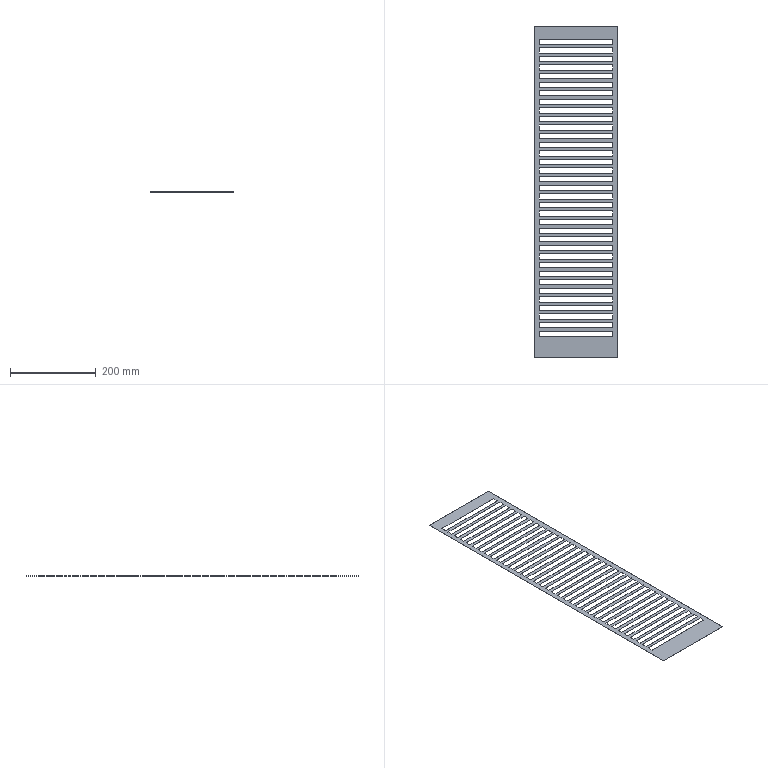Part | SolidWorks | features FlatPattern 1, ICE 1, SMBaseFlange 1, SheetMetal 1 | 1 solid | 146 faces | box 194.4 x 773 x 0.26 mm | volume 19811 mm3 | plane 146